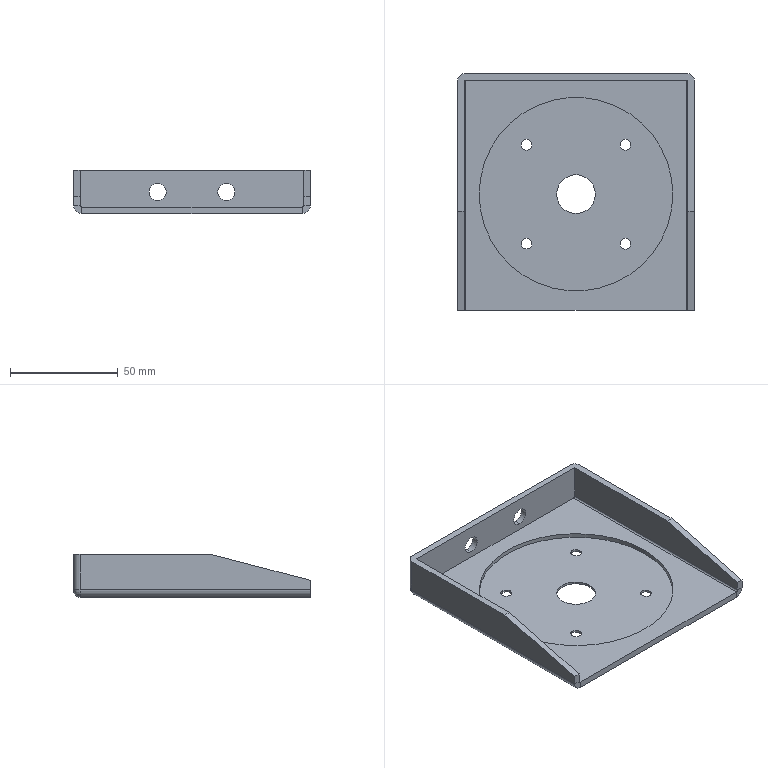Part | SolidWorks | features ICE 5, MirrorPattern 2, Cut 1, EdgeFlange 1, Fillet 1, FlatPattern 1, SMBaseFlange 1, SheetMetal 1 | 1 solid | 42 faces | box 110 x 110 x 20 mm | volume 36896 mm3 | cylinder 23 | plane 17 | torus 2 | commonest cylinder face diameters 5 x8 8 x4 6 x3 1.473 x2 7.473 x2 18 x2
STEP:
#1=CARTESIAN_POINT('',(-45.,-1.,-2.));
#2=VERTEX_POINT('',#1);
#3=CARTESIAN_POINT('',(45.,-1.,-2.));
#4=VERTEX_POINT('',#3);
#5=CARTESIAN_POINT('',(0.,-1.,-2.));
#6=DIRECTION('',(0.,0.,1.));
#7=DIRECTION('',(1.,0.,0.));
#8=AXIS2_PLACEMENT_3D('',#5,#6,#7);
#9=CIRCLE('',#8,45.);
#10=EDGE_CURVE('',#2,#4,#9,.T.);
#11=ORIENTED_EDGE('',*,*,#10,.F.);
#12=CARTESIAN_POINT('',(-45.,-1.,0.));
#13=VERTEX_POINT('',#12);
#14=CARTESIAN_POINT('',(-45.,-1.,-2.));
#15=DIRECTION('',(0.,0.,1.));
#16=VECTOR('',#15,1000.);
#17=LINE('',#14,#16);
#18=EDGE_CURVE('',#2,#13,#17,.T.);
#19=ORIENTED_EDGE('',*,*,#18,.T.);
#20=CARTESIAN_POINT('',(45.,-1.,0.));
#21=VERTEX_POINT('',#20);
#22=CARTESIAN_POINT('',(0.,-1.,0.));
#23=DIRECTION('',(0.,0.,1.));
#24=DIRECTION('',(1.,0.,0.));
#25=AXIS2_PLACEMENT_3D('',#22,#23,#24);
#26=CIRCLE('',#25,45.);
#27=EDGE_CURVE('',#13,#21,#26,.T.);
#28=ORIENTED_EDGE('',*,*,#27,.T.);
#29=CARTESIAN_POINT('',(45.,-1.,-2.));
#30=DIRECTION('',(0.,0.,1.));
#31=VECTOR('',#30,1000.);
#32=LINE('',#29,#31);
#33=EDGE_CURVE('',#4,#21,#32,.T.);
#34=ORIENTED_EDGE('',*,*,#33,.F.);
#35=EDGE_LOOP('',(#11,#19,#28,#34));
#36=FACE_OUTER_BOUND('',#35,.T.);
#37=CARTESIAN_POINT('',(0.,-1.,-2.));
#38=DIRECTION('',(0.,0.,1.));
#39=DIRECTION('',(1.,0.,0.));
#40=AXIS2_PLACEMENT_3D('',#37,#38,#39);
#41=CYLINDRICAL_SURFACE('',#40,45.);
#42=ADVANCED_FACE('',(#36),#41,.F.);
#43=CARTESIAN_POINT('',(-16.,52.,3.));
#44=VERTEX_POINT('',#43);
#45=CARTESIAN_POINT('',(-16.,52.,11.));
#46=VERTEX_POINT('',#45);
#47=CARTESIAN_POINT('',(-16.,52.,7.));
#48=DIRECTION('',(0.,1.,0.));
#49=DIRECTION('',(0.,0.,1.));
#50=AXIS2_PLACEMENT_3D('',#47,#48,#49);
#51=CIRCLE('',#50,4.);
#52=EDGE_CURVE('',#44,#46,#51,.T.);
#53=ORIENTED_EDGE('',*,*,#52,.F.);
#54=CARTESIAN_POINT('',(-16.,55.,3.));
#55=VERTEX_POINT('',#54);
#56=CARTESIAN_POINT('',(-16.,52.,3.));
#57=DIRECTION('',(0.,1.,0.));
#58=VECTOR('',#57,1000.);
#59=LINE('',#56,#58);
#60=EDGE_CURVE('',#44,#55,#59,.T.);
#61=ORIENTED_EDGE('',*,*,#60,.T.);
#62=CARTESIAN_POINT('',(-16.,55.,11.));
#63=VERTEX_POINT('',#62);
#64=CARTESIAN_POINT('',(-16.,55.,7.));
#65=DIRECTION('',(0.,1.,0.));
#66=DIRECTION('',(0.,0.,1.));
#67=AXIS2_PLACEMENT_3D('',#64,#65,#66);
#68=CIRCLE('',#67,4.);
#69=EDGE_CURVE('',#55,#63,#68,.T.);
#70=ORIENTED_EDGE('',*,*,#69,.T.);
#71=CARTESIAN_POINT('',(-16.,52.,11.));
#72=DIRECTION('',(0.,1.,0.));
#73=VECTOR('',#72,1000.);
#74=LINE('',#71,#73);
#75=EDGE_CURVE('',#46,#63,#74,.T.);
#76=ORIENTED_EDGE('',*,*,#75,.F.);
#77=EDGE_LOOP('',(#53,#61,#70,#76));
#78=FACE_OUTER_BOUND('',#77,.T.);
#79=CARTESIAN_POINT('',(-16.,52.,7.));
#80=DIRECTION('',(0.,1.,0.));
#81=DIRECTION('',(0.,0.,1.));
#82=AXIS2_PLACEMENT_3D('',#79,#80,#81);
#83=CYLINDRICAL_SURFACE('',#82,4.);
#84=ADVANCED_FACE('',(#78),#83,.F.);
#85=CARTESIAN_POINT('',(16.,52.,3.));
#86=VERTEX_POINT('',#85);
#87=CARTESIAN_POINT('',(16.,52.,11.));
#88=VERTEX_POINT('',#87);
#89=CARTESIAN_POINT('',(16.,52.,7.));
#90=DIRECTION('',(0.,1.,0.));
#91=DIRECTION('',(0.,0.,1.));
#92=AXIS2_PLACEMENT_3D('',#89,#90,#91);
#93=CIRCLE('',#92,4.);
#94=EDGE_CURVE('',#86,#88,#93,.T.);
#95=ORIENTED_EDGE('',*,*,#94,.F.);
#96=CARTESIAN_POINT('',(16.,55.,3.));
#97=VERTEX_POINT('',#96);
#98=CARTESIAN_POINT('',(16.,52.,3.));
#99=DIRECTION('',(0.,1.,0.));
#100=VECTOR('',#99,1000.);
#101=LINE('',#98,#100);
#102=EDGE_CURVE('',#86,#97,#101,.T.);
#103=ORIENTED_EDGE('',*,*,#102,.T.);
#104=CARTESIAN_POINT('',(16.,55.,11.));
#105=VERTEX_POINT('',#104);
#106=CARTESIAN_POINT('',(16.,55.,7.));
#107=DIRECTION('',(0.,1.,0.));
#108=DIRECTION('',(0.,0.,1.));
#109=AXIS2_PLACEMENT_3D('',#106,#107,#108);
#110=CIRCLE('',#109,4.);
#111=EDGE_CURVE('',#97,#105,#110,.T.);
#112=ORIENTED_EDGE('',*,*,#111,.T.);
#113=CARTESIAN_POINT('',(16.,52.,11.));
#114=DIRECTION('',(0.,1.,0.));
#115=VECTOR('',#114,1000.);
#116=LINE('',#113,#115);
#117=EDGE_CURVE('',#88,#105,#116,.T.);
#118=ORIENTED_EDGE('',*,*,#117,.F.);
#119=EDGE_LOOP('',(#95,#103,#112,#118));
#120=FACE_OUTER_BOUND('',#119,.T.);
#121=CARTESIAN_POINT('',(16.,52.,7.));
#122=DIRECTION('',(0.,1.,0.));
#123=DIRECTION('',(0.,0.,1.));
#124=AXIS2_PLACEMENT_3D('',#121,#122,#123);
#125=CYLINDRICAL_SURFACE('',#124,4.);
#126=ADVANCED_FACE('',(#120),#125,.F.);
#127=CARTESIAN_POINT('',(20.451,-24.011,-3.));
#128=VERTEX_POINT('',#127);
#129=CARTESIAN_POINT('',(25.451,-24.011,-3.));
#130=VERTEX_POINT('',#129);
#131=CARTESIAN_POINT('',(22.951,-24.011,-3.));
#132=DIRECTION('',(0.,0.,1.));
#133=DIRECTION('',(-1.,0.,0.));
#134=AXIS2_PLACEMENT_3D('',#131,#132,#133);
#135=CIRCLE('',#134,2.5);
#136=EDGE_CURVE('',#128,#130,#135,.T.);
#137=ORIENTED_EDGE('',*,*,#136,.F.);
#138=CARTESIAN_POINT('',(20.451,-24.011,-2.));
#139=VERTEX_POINT('',#138);
#140=CARTESIAN_POINT('',(20.451,-24.011,-3.));
#141=DIRECTION('',(0.,0.,1.));
#142=VECTOR('',#141,1000.);
#143=LINE('',#140,#142);
#144=EDGE_CURVE('',#128,#139,#143,.T.);
#145=ORIENTED_EDGE('',*,*,#144,.T.);
#146=CARTESIAN_POINT('',(25.451,-24.011,-2.));
#147=VERTEX_POINT('',#146);
#148=CARTESIAN_POINT('',(22.951,-24.011,-2.));
#149=DIRECTION('',(0.,0.,-1.));
#150=DIRECTION('',(1.,0.,0.));
#151=AXIS2_PLACEMENT_3D('',#148,#149,#150);
#152=CIRCLE('',#151,2.5);
#153=EDGE_CURVE('',#147,#139,#152,.T.);
#154=ORIENTED_EDGE('',*,*,#153,.F.);
#155=CARTESIAN_POINT('',(25.451,-24.011,-3.));
#156=DIRECTION('',(0.,0.,1.));
#157=VECTOR('',#156,1000.);
#158=LINE('',#155,#157);
#159=EDGE_CURVE('',#130,#147,#158,.T.);
#160=ORIENTED_EDGE('',*,*,#159,.F.);
#161=EDGE_LOOP('',(#137,#145,#154,#160));
#162=FACE_OUTER_BOUND('',#161,.T.);
#163=CARTESIAN_POINT('',(22.951,-24.011,-3.));
#164=DIRECTION('',(0.,0.,1.));
#165=DIRECTION('',(1.,0.,0.));
#166=AXIS2_PLACEMENT_3D('',#163,#164,#165);
#167=CYLINDRICAL_SURFACE('',#166,2.5);
#168=ADVANCED_FACE('',(#162),#167,.F.);
#169=CARTESIAN_POINT('',(-25.481,-23.981,-3.));
#170=VERTEX_POINT('',#169);
#171=CARTESIAN_POINT('',(-20.481,-23.981,-3.));
#172=VERTEX_POINT('',#171);
#173=CARTESIAN_POINT('',(-22.981,-23.981,-3.));
#174=DIRECTION('',(0.,0.,1.));
#175=DIRECTION('',(-1.,0.,0.));
#176=AXIS2_PLACEMENT_3D('',#173,#174,#175);
#177=CIRCLE('',#176,2.5);
#178=EDGE_CURVE('',#170,#172,#177,.T.);
#179=ORIENTED_EDGE('',*,*,#178,.F.);
#180=CARTESIAN_POINT('',(-25.481,-23.981,-2.));
#181=VERTEX_POINT('',#180);
#182=CARTESIAN_POINT('',(-25.481,-23.981,-3.));
#183=DIRECTION('',(0.,0.,1.));
#184=VECTOR('',#183,1000.);
#185=LINE('',#182,#184);
#186=EDGE_CURVE('',#170,#181,#185,.T.);
#187=ORIENTED_EDGE('',*,*,#186,.T.);
#188=CARTESIAN_POINT('',(-20.481,-23.981,-2.));
#189=VERTEX_POINT('',#188);
#190=CARTESIAN_POINT('',(-22.981,-23.981,-2.));
#191=DIRECTION('',(0.,0.,-1.));
#192=DIRECTION('',(1.,0.,0.));
#193=AXIS2_PLACEMENT_3D('',#190,#191,#192);
#194=CIRCLE('',#193,2.5);
#195=EDGE_CURVE('',#189,#181,#194,.T.);
#196=ORIENTED_EDGE('',*,*,#195,.F.);
#197=CARTESIAN_POINT('',(-20.481,-23.981,-3.));
#198=DIRECTION('',(0.,0.,1.));
#199=VECTOR('',#198,1000.);
#200=LINE('',#197,#199);
#201=EDGE_CURVE('',#172,#189,#200,.T.);
#202=ORIENTED_EDGE('',*,*,#201,.F.);
#203=EDGE_LOOP('',(#179,#187,#196,#202));
#204=FACE_OUTER_BOUND('',#203,.T.);
#205=CARTESIAN_POINT('',(-22.981,-23.981,-3.));
#206=DIRECTION('',(0.,0.,1.));
#207=DIRECTION('',(1.,0.,0.));
#208=AXIS2_PLACEMENT_3D('',#205,#206,#207);
#209=CYLINDRICAL_SURFACE('',#208,2.5);
#210=ADVANCED_FACE('',(#204),#209,.F.);
#211=CARTESIAN_POINT('',(-25.481,21.981,-3.));
#212=VERTEX_POINT('',#211);
#213=CARTESIAN_POINT('',(-20.481,21.981,-3.));
#214=VERTEX_POINT('',#213);
#215=CARTESIAN_POINT('',(-22.981,21.981,-3.));
#216=DIRECTION('',(0.,0.,1.));
#217=DIRECTION('',(1.,0.,0.));
#218=AXIS2_PLACEMENT_3D('',#215,#216,#217);
#219=CIRCLE('',#218,2.5);
#220=EDGE_CURVE('',#212,#214,#219,.T.);
#221=ORIENTED_EDGE('',*,*,#220,.F.);
#222=CARTESIAN_POINT('',(-25.481,21.981,-2.));
#223=VERTEX_POINT('',#222);
#224=CARTESIAN_POINT('',(-25.481,21.981,-3.));
#225=DIRECTION('',(0.,0.,1.));
#226=VECTOR('',#225,1000.);
#227=LINE('',#224,#226);
#228=EDGE_CURVE('',#212,#223,#227,.T.);
#229=ORIENTED_EDGE('',*,*,#228,.T.);
#230=CARTESIAN_POINT('',(-20.481,21.981,-2.));
#231=VERTEX_POINT('',#230);
#232=CARTESIAN_POINT('',(-22.981,21.981,-2.));
#233=DIRECTION('',(0.,0.,-1.));
#234=DIRECTION('',(1.,0.,0.));
#235=AXIS2_PLACEMENT_3D('',#232,#233,#234);
#236=CIRCLE('',#235,2.5);
#237=EDGE_CURVE('',#231,#223,#236,.T.);
#238=ORIENTED_EDGE('',*,*,#237,.F.);
#239=CARTESIAN_POINT('',(-20.481,21.981,-3.));
#240=DIRECTION('',(0.,0.,1.));
#241=VECTOR('',#240,1000.);
#242=LINE('',#239,#241);
#243=EDGE_CURVE('',#214,#231,#242,.T.);
#244=ORIENTED_EDGE('',*,*,#243,.F.);
#245=EDGE_LOOP('',(#221,#229,#238,#244));
#246=FACE_OUTER_BOUND('',#245,.T.);
#247=CARTESIAN_POINT('',(-22.981,21.981,-3.));
#248=DIRECTION('',(0.,0.,1.));
#249=DIRECTION('',(1.,0.,0.));
#250=AXIS2_PLACEMENT_3D('',#247,#248,#249);
#251=CYLINDRICAL_SURFACE('',#250,2.5);
#252=ADVANCED_FACE('',(#246),#251,.F.);
#253=CARTESIAN_POINT('',(20.451,22.011,-3.));
#254=VERTEX_POINT('',#253);
#255=CARTESIAN_POINT('',(25.451,22.011,-3.));
#256=VERTEX_POINT('',#255);
#257=CARTESIAN_POINT('',(22.951,22.011,-3.));
#258=DIRECTION('',(0.,0.,1.));
#259=DIRECTION('',(1.,0.,0.));
#260=AXIS2_PLACEMENT_3D('',#257,#258,#259);
#261=CIRCLE('',#260,2.5);
#262=EDGE_CURVE('',#254,#256,#261,.T.);
#263=ORIENTED_EDGE('',*,*,#262,.F.);
#264=CARTESIAN_POINT('',(20.451,22.011,-2.));
#265=VERTEX_POINT('',#264);
#266=CARTESIAN_POINT('',(20.451,22.011,-3.));
#267=DIRECTION('',(0.,0.,1.));
#268=VECTOR('',#267,1000.);
#269=LINE('',#266,#268);
#270=EDGE_CURVE('',#254,#265,#269,.T.);
#271=ORIENTED_EDGE('',*,*,#270,.T.);
#272=CARTESIAN_POINT('',(25.451,22.011,-2.));
#273=VERTEX_POINT('',#272);
#274=CARTESIAN_POINT('',(22.951,22.011,-2.));
#275=DIRECTION('',(0.,0.,-1.));
#276=DIRECTION('',(1.,0.,0.));
#277=AXIS2_PLACEMENT_3D('',#274,#275,#276);
#278=CIRCLE('',#277,2.5);
#279=EDGE_CURVE('',#273,#265,#278,.T.);
#280=ORIENTED_EDGE('',*,*,#279,.F.);
#281=CARTESIAN_POINT('',(25.451,22.011,-3.));
#282=DIRECTION('',(0.,0.,1.));
#283=VECTOR('',#282,1000.);
#284=LINE('',#281,#283);
#285=EDGE_CURVE('',#256,#273,#284,.T.);
#286=ORIENTED_EDGE('',*,*,#285,.F.);
#287=EDGE_LOOP('',(#263,#271,#280,#286));
#288=FACE_OUTER_BOUND('',#287,.T.);
#289=CARTESIAN_POINT('',(22.951,22.011,-3.));
#290=DIRECTION('',(0.,0.,1.));
#291=DIRECTION('',(1.,0.,0.));
#292=AXIS2_PLACEMENT_3D('',#289,#290,#291);
#293=CYLINDRICAL_SURFACE('',#292,2.5);
#294=ADVANCED_FACE('',(#288),#293,.F.);
#295=CARTESIAN_POINT('',(-9.,-1.,-3.));
#296=VERTEX_POINT('',#295);
#297=CARTESIAN_POINT('',(9.,-1.,-3.));
#298=VERTEX_POINT('',#297);
#299=CARTESIAN_POINT('',(0.,-1.,-3.));
#300=DIRECTION('',(0.,0.,1.));
#301=DIRECTION('',(1.,0.,0.));
#302=AXIS2_PLACEMENT_3D('',#299,#300,#301);
#303=CIRCLE('',#302,9.);
#304=EDGE_CURVE('',#296,#298,#303,.T.);
#305=ORIENTED_EDGE('',*,*,#304,.F.);
#306=CARTESIAN_POINT('',(-9.,-1.,-2.));
#307=VERTEX_POINT('',#306);
#308=CARTESIAN_POINT('',(-9.,-1.,-3.));
#309=DIRECTION('',(0.,0.,1.));
#310=VECTOR('',#309,1000.);
#311=LINE('',#308,#310);
#312=EDGE_CURVE('',#296,#307,#311,.T.);
#313=ORIENTED_EDGE('',*,*,#312,.T.);
#314=CARTESIAN_POINT('',(9.,-1.,-2.));
#315=VERTEX_POINT('',#314);
#316=CARTESIAN_POINT('',(0.,-1.,-2.));
#317=DIRECTION('',(0.,0.,-1.));
#318=DIRECTION('',(1.,0.,0.));
#319=AXIS2_PLACEMENT_3D('',#316,#317,#318);
#320=CIRCLE('',#319,9.);
#321=EDGE_CURVE('',#315,#307,#320,.T.);
#322=ORIENTED_EDGE('',*,*,#321,.F.);
#323=CARTESIAN_POINT('',(9.,-1.,-3.));
#324=DIRECTION('',(0.,0.,1.));
#325=VECTOR('',#324,1000.);
#326=LINE('',#323,#325);
#327=EDGE_CURVE('',#298,#315,#326,.T.);
#328=ORIENTED_EDGE('',*,*,#327,.F.);
#329=EDGE_LOOP('',(#305,#313,#322,#328));
#330=FACE_OUTER_BOUND('',#329,.T.);
#331=CARTESIAN_POINT('',(0.,-1.,-3.));
#332=DIRECTION('',(0.,0.,1.));
#333=DIRECTION('',(1.,0.,0.));
#334=AXIS2_PLACEMENT_3D('',#331,#332,#333);
#335=CYLINDRICAL_SURFACE('',#334,9.);
#336=ADVANCED_FACE('',(#330),#335,.F.);
#337=ORIENTED_EDGE('',*,*,#312,.F.);
#338=CARTESIAN_POINT('',(0.,-1.,-3.));
#339=DIRECTION('',(0.,0.,1.));
#340=DIRECTION('',(1.,0.,0.));
#341=AXIS2_PLACEMENT_3D('',#338,#339,#340);
#342=CIRCLE('',#341,9.);
#343=EDGE_CURVE('',#298,#296,#342,.T.);
#344=ORIENTED_EDGE('',*,*,#343,.F.);
#345=ORIENTED_EDGE('',*,*,#327,.T.);
#346=CARTESIAN_POINT('',(0.,-1.,-2.));
#347=DIRECTION('',(0.,0.,-1.));
#348=DIRECTION('',(1.,0.,0.));
#349=AXIS2_PLACEMENT_3D('',#346,#347,#348);
#350=CIRCLE('',#349,9.);
#351=EDGE_CURVE('',#307,#315,#350,.T.);
#352=ORIENTED_EDGE('',*,*,#351,.F.);
#353=EDGE_LOOP('',(#337,#344,#345,#352));
#354=FACE_OUTER_BOUND('',#353,.T.);
#355=CARTESIAN_POINT('',(0.,-1.,-3.));
#356=DIRECTION('',(0.,0.,1.));
#357=DIRECTION('',(1.,0.,0.));
#358=AXIS2_PLACEMENT_3D('',#355,#356,#357);
#359=CYLINDRICAL_SURFACE('',#358,9.);
#360=ADVANCED_FACE('',(#354),#359,.F.);
#361=ORIENTED_EDGE('',*,*,#270,.F.);
#362=CARTESIAN_POINT('',(22.951,22.011,-3.));
#363=DIRECTION('',(0.,0.,1.));
#364=DIRECTION('',(1.,0.,0.));
#365=AXIS2_PLACEMENT_3D('',#362,#363,#364);
#366=CIRCLE('',#365,2.5);
#367=EDGE_CURVE('',#256,#254,#366,.T.);
#368=ORIENTED_EDGE('',*,*,#367,.F.);
#369=ORIENTED_EDGE('',*,*,#285,.T.);
#370=CARTESIAN_POINT('',(22.951,22.011,-2.));
#371=DIRECTION('',(0.,0.,-1.));
#372=DIRECTION('',(1.,0.,0.));
#373=AXIS2_PLACEMENT_3D('',#370,#371,#372);
#374=CIRCLE('',#373,2.5);
#375=EDGE_CURVE('',#265,#273,#374,.T.);
#376=ORIENTED_EDGE('',*,*,#375,.F.);
#377=EDGE_LOOP('',(#361,#368,#369,#376));
#378=FACE_OUTER_BOUND('',#377,.T.);
#379=CARTESIAN_POINT('',(22.951,22.011,-3.));
#380=DIRECTION('',(0.,0.,1.));
#381=DIRECTION('',(1.,0.,0.));
#382=AXIS2_PLACEMENT_3D('',#379,#380,#381);
#383=CYLINDRICAL_SURFACE('',#382,2.5);
#384=ADVANCED_FACE('',(#378),#383,.F.);
#385=ORIENTED_EDGE('',*,*,#228,.F.);
#386=CARTESIAN_POINT('',(-22.981,21.981,-3.));
#387=DIRECTION('',(0.,0.,1.));
#388=DIRECTION('',(1.,0.,0.));
#389=AXIS2_PLACEMENT_3D('',#386,#387,#388);
#390=CIRCLE('',#389,2.5);
#391=EDGE_CURVE('',#214,#212,#390,.T.);
#392=ORIENTED_EDGE('',*,*,#391,.F.);
#393=ORIENTED_EDGE('',*,*,#243,.T.);
#394=CARTESIAN_POINT('',(-22.981,21.981,-2.));
#395=DIRECTION('',(0.,0.,-1.));
#396=DIRECTION('',(1.,0.,0.));
#397=AXIS2_PLACEMENT_3D('',#394,#395,#396);
#398=CIRCLE('',#397,2.5);
#399=EDGE_CURVE('',#223,#231,#398,.T.);
#400=ORIENTED_EDGE('',*,*,#399,.F.);
#401=EDGE_LOOP('',(#385,#392,#393,#400));
#402=FACE_OUTER_BOUND('',#401,.T.);
#403=CARTESIAN_POINT('',(-22.981,21.981,-3.));
#404=DIRECTION('',(0.,0.,1.));
#405=DIRECTION('',(1.,0.,0.));
#406=AXIS2_PLACEMENT_3D('',#403,#404,#405);
#407=CYLINDRICAL_SURFACE('',#406,2.5);
#408=ADVANCED_FACE('',(#402),#407,.F.);
#409=ORIENTED_EDGE('',*,*,#186,.F.);
#410=CARTESIAN_POINT('',(-22.981,-23.981,-3.));
#411=DIRECTION('',(0.,0.,1.));
#412=DIRECTION('',(-1.,0.,0.));
#413=AXIS2_PLACEMENT_3D('',#410,#411,#412);
#414=CIRCLE('',#413,2.5);
#415=EDGE_CURVE('',#172,#170,#414,.T.);
#416=ORIENTED_EDGE('',*,*,#415,.F.);
#417=ORIENTED_EDGE('',*,*,#201,.T.);
#418=CARTESIAN_POINT('',(-22.981,-23.981,-2.));
#419=DIRECTION('',(0.,0.,-1.));
#420=DIRECTION('',(1.,0.,0.));
#421=AXIS2_PLACEMENT_3D('',#418,#419,#420);
#422=CIRCLE('',#421,2.5);
#423=EDGE_CURVE('',#181,#189,#422,.T.);
#424=ORIENTED_EDGE('',*,*,#423,.F.);
#425=EDGE_LOOP('',(#409,#416,#417,#424));
#426=FACE_OUTER_BOUND('',#425,.T.);
#427=CARTESIAN_POINT('',(-22.981,-23.981,-3.));
#428=DIRECTION('',(0.,0.,1.));
#429=DIRECTION('',(1.,0.,0.));
#430=AXIS2_PLACEMENT_3D('',#427,#428,#429);
#431=CYLINDRICAL_SURFACE('',#430,2.5);
#432=ADVANCED_FACE('',(#426),#431,.F.);
#433=ORIENTED_EDGE('',*,*,#144,.F.);
#434=CARTESIAN_POINT('',(22.951,-24.011,-3.));
#435=DIRECTION('',(0.,0.,1.));
#436=DIRECTION('',(-1.,0.,0.));
#437=AXIS2_PLACEMENT_3D('',#434,#435,#436);
#438=CIRCLE('',#437,2.5);
#439=EDGE_CURVE('',#130,#128,#438,.T.);
#440=ORIENTED_EDGE('',*,*,#439,.F.);
#441=ORIENTED_EDGE('',*,*,#159,.T.);
#442=CARTESIAN_POINT('',(22.951,-24.011,-2.));
#443=DIRECTION('',(0.,0.,-1.));
#444=DIRECTION('',(1.,0.,0.));
#445=AXIS2_PLACEMENT_3D('',#442,#443,#444);
#446=CIRCLE('',#445,2.5);
#447=EDGE_CURVE('',#139,#147,#446,.T.);
#448=ORIENTED_EDGE('',*,*,#447,.F.);
#449=EDGE_LOOP('',(#433,#440,#441,#448));
#450=FACE_OUTER_BOUND('',#449,.T.);
#451=CARTESIAN_POINT('',(22.951,-24.011,-3.));
#452=DIRECTION('',(0.,0.,1.));
#453=DIRECTION('',(1.,0.,0.));
#454=AXIS2_PLACEMENT_3D('',#451,#452,#453);
#455=CYLINDRICAL_SURFACE('',#454,2.5);
#456=ADVANCED_FACE('',(#450),#455,.F.);
#457=CARTESIAN_POINT('',(-52.,52.,17.));
#458=VERTEX_POINT('',#457);
#459=CARTESIAN_POINT('',(-52.,-9.,17.));
#460=VERTEX_POINT('',#459);
#461=CARTESIAN_POINT('',(-52.,0.,17.));
#462=DIRECTION('',(0.,-1.,0.));
#463=VECTOR('',#462,1000.);
#464=LINE('',#461,#463);
#465=EDGE_CURVE('',#458,#460,#464,.T.);
#466=ORIENTED_EDGE('',*,*,#465,.T.);
#467=CARTESIAN_POINT('',(-52.,-55.,5.));
#468=VERTEX_POINT('',#467);
#469=CARTESIAN_POINT('',(-52.,-4.726,18.115));
#470=DIRECTION('',(0.,-0.9676,-0.2524));
#471=VECTOR('',#470,1000.);
#472=LINE('',#469,#471);
#473=EDGE_CURVE('',#460,#468,#472,.T.);
#474=ORIENTED_EDGE('',*,*,#473,.T.);
#475=CARTESIAN_POINT('',(-52.,-55.,0.7366));
#476=VERTEX_POINT('',#475);
#477=CARTESIAN_POINT('',(-52.,-55.,0.));
#478=DIRECTION('',(0.,0.,-1.));
#479=VECTOR('',#478,1000.);
#480=LINE('',#477,#479);
#481=EDGE_CURVE('',#468,#476,#480,.T.);
#482=ORIENTED_EDGE('',*,*,#481,.T.);
#483=CARTESIAN_POINT('',(-52.,52.,0.7366));
#484=VERTEX_POINT('',#483);
#485=CARTESIAN_POINT('',(-52.,55.,0.7366));
#486=DIRECTION('',(0.,-1.,0.));
#487=VECTOR('',#486,1000.);
#488=LINE('',#485,#487);
#489=EDGE_CURVE('',#484,#476,#488,.T.);
#490=ORIENTED_EDGE('',*,*,#489,.F.);
#491=CARTESIAN_POINT('',(-52.,52.,0.7366));
#492=DIRECTION('',(0.,0.,1.));
#493=VECTOR('',#492,1000.);
#494=LINE('',#491,#493);
#495=EDGE_CURVE('',#484,#458,#494,.T.);
#496=ORIENTED_EDGE('',*,*,#495,.T.);
#497=EDGE_LOOP('',(#466,#474,#482,#490,#496));
#498=FACE_OUTER_BOUND('',#497,.T.);
#499=CARTESIAN_POINT('',(-52.,0.,0.));
#500=DIRECTION('',(1.,0.,0.));
#501=DIRECTION('',(0.,0.,1.));
#502=AXIS2_PLACEMENT_3D('',#499,#500,#501);
#503=PLANE('',#502);
#504=ADVANCED_FACE('',(#498),#503,.T.);
#505=CARTESIAN_POINT('',(-55.,-9.,17.));
#506=VERTEX_POINT('',#505);
#507=CARTESIAN_POINT('',(-45.,-9.,17.));
#508=DIRECTION('',(-1.,0.,0.));
#509=VECTOR('',#508,1000.);
#510=LINE('',#507,#509);
#511=EDGE_CURVE('',#460,#506,#510,.T.);
#512=ORIENTED_EDGE('',*,*,#511,.F.);
#513=ORIENTED_EDGE('',*,*,#465,.F.);
#514=CARTESIAN_POINT('',(52.,52.,17.));
#515=VERTEX_POINT('',#514);
#516=CARTESIAN_POINT('',(-52.,52.,17.));
#517=DIRECTION('',(1.,0.,0.));
#518=VECTOR('',#517,1000.);
#519=LINE('',#516,#518);
#520=EDGE_CURVE('',#458,#515,#519,.T.);
#521=ORIENTED_EDGE('',*,*,#520,.T.);
#522=CARTESIAN_POINT('',(52.,-9.,17.));
#523=VERTEX_POINT('',#522);
#524=CARTESIAN_POINT('',(52.,-55.,17.));
#525=DIRECTION('',(0.,-1.,0.));
#526=VECTOR('',#525,1000.);
#527=LINE('',#524,#526);
#528=EDGE_CURVE('',#515,#523,#527,.T.);
#529=ORIENTED_EDGE('',*,*,#528,.T.);
#530=CARTESIAN_POINT('',(55.,-9.,17.));
#531=VERTEX_POINT('',#530);
#532=CARTESIAN_POINT('',(55.,-9.,17.));
#533=DIRECTION('',(1.,0.,0.));
#534=VECTOR('',#533,1000.);
#535=LINE('',#532,#534);
#536=EDGE_CURVE('',#523,#531,#535,.T.);
#537=ORIENTED_EDGE('',*,*,#536,.T.);
#538=CARTESIAN_POINT('',(55.,52.,17.));
#539=VERTEX_POINT('',#538);
#540=CARTESIAN_POINT('',(55.,0.,17.));
#541=DIRECTION('',(0.,-1.,0.));
#542=VECTOR('',#541,1000.);
#543=LINE('',#540,#542);
#544=EDGE_CURVE('',#539,#531,#543,.T.);
#545=ORIENTED_EDGE('',*,*,#544,.F.);
#546=CARTESIAN_POINT('',(52.,55.,17.));
#547=VERTEX_POINT('',#546);
#548=CARTESIAN_POINT('',(52.,52.,17.));
#549=DIRECTION('',(0.,0.,1.));
#550=DIRECTION('',(-1.,0.,0.));
#551=AXIS2_PLACEMENT_3D('',#548,#549,#550);
#552=CIRCLE('',#551,3.);
#553=EDGE_CURVE('',#539,#547,#552,.T.);
#554=ORIENTED_EDGE('',*,*,#553,.T.);
#555=CARTESIAN_POINT('',(-52.,55.,17.));
#556=VERTEX_POINT('',#555);
#557=CARTESIAN_POINT('',(55.,55.,17.));
#558=DIRECTION('',(-1.,0.,0.));
#559=VECTOR('',#558,1000.);
#560=LINE('',#557,#559);
#561=EDGE_CURVE('',#547,#556,#560,.T.);
#562=ORIENTED_EDGE('',*,*,#561,.T.);
#563=CARTESIAN_POINT('',(-55.,52.,17.));
#564=VERTEX_POINT('',#563);
#565=CARTESIAN_POINT('',(-52.,52.,17.));
#566=DIRECTION('',(0.,0.,1.));
#567=DIRECTION('',(-1.,0.,0.));
#568=AXIS2_PLACEMENT_3D('',#565,#566,#567);
#569=CIRCLE('',#568,3.);
#570=EDGE_CURVE('',#556,#564,#569,.T.);
#571=ORIENTED_EDGE('',*,*,#570,.T.);
#572=CARTESIAN_POINT('',(-55.,-55.,17.));
#573=DIRECTION('',(0.,-1.,0.));
#574=VECTOR('',#573,1000.);
#575=LINE('',#572,#574);
#576=EDGE_CURVE('',#564,#506,#575,.T.);
#577=ORIENTED_EDGE('',*,*,#576,.T.);
#578=EDGE_LOOP('',(#512,#513,#521,#529,#537,#545,#554,#562,#571,#577));
#579=FACE_OUTER_BOUND('',#578,.T.);
#580=CARTESIAN_POINT('',(55.,-55.,17.));
#581=DIRECTION('',(0.,0.,-1.));
#582=DIRECTION('',(-1.,0.,0.));
#583=AXIS2_PLACEMENT_3D('',#580,#581,#582);
#584=PLANE('',#583);
#585=ADVANCED_FACE('',(#579),#584,.F.);
#586=ORIENTED_EDGE('',*,*,#481,.F.);
#587=CARTESIAN_POINT('',(-55.,-55.,5.));
#588=VERTEX_POINT('',#587);
#589=CARTESIAN_POINT('',(-45.,-55.,5.));
#590=DIRECTION('',(-1.,0.,0.));
#591=VECTOR('',#590,1000.);
#592=LINE('',#589,#591);
#593=EDGE_CURVE('',#468,#588,#592,.T.);
#594=ORIENTED_EDGE('',*,*,#593,.T.);
#595=CARTESIAN_POINT('',(-55.,-55.,0.7366));
#596=VERTEX_POINT('',#595);
#597=CARTESIAN_POINT('',(-55.,-55.,0.));
#598=DIRECTION('',(0.,0.,-1.));
#599=VECTOR('',#598,1000.);
#600=LINE('',#597,#599);
#601=EDGE_CURVE('',#588,#596,#600,.T.);
#602=ORIENTED_EDGE('',*,*,#601,.T.);
#603=CARTESIAN_POINT('',(-52.,-55.,0.7366));
#604=DIRECTION('',(-1.,0.,0.));
#605=VECTOR('',#604,1000.);
#606=LINE('',#603,#605);
#607=EDGE_CURVE('',#476,#596,#606,.T.);
#608=ORIENTED_EDGE('',*,*,#607,.F.);
#609=EDGE_LOOP('',(#586,#594,#602,#608));
#610=FACE_OUTER_BOUND('',#609,.T.);
#611=CARTESIAN_POINT('',(-55.,-55.,0.));
#612=DIRECTION('',(0.,-1.,0.));
#613=DIRECTION('',(0.,0.,-1.));
#614=AXIS2_PLACEMENT_3D('',#611,#612,#613);
#615=PLANE('',#614);
#616=ADVANCED_FACE('',(#610),#615,.T.);
#617=CARTESIAN_POINT('',(-55.,-55.,5.));
#618=DIRECTION('',(0.,0.9676,0.2524));
#619=VECTOR('',#618,1000.);
#620=LINE('',#617,#619);
#621=EDGE_CURVE('',#588,#506,#620,.T.);
#622=ORIENTED_EDGE('',*,*,#621,.T.);
#623=ORIENTED_EDGE('',*,*,#576,.F.);
#624=CARTESIAN_POINT('',(-55.,52.,0.7366));
#625=VERTEX_POINT('',#624);
#626=CARTESIAN_POINT('',(-55.,52.,0.7366));
#627=DIRECTION('',(0.,0.,-1.));
#628=VECTOR('',#627,1000.);
#629=LINE('',#626,#628);
#630=EDGE_CURVE('',#564,#625,#629,.T.);
#631=ORIENTED_EDGE('',*,*,#630,.T.);
#632=CARTESIAN_POINT('',(-55.,55.,0.7366));
#633=DIRECTION('',(0.,1.,0.));
#634=VECTOR('',#633,1000.);
#635=LINE('',#632,#634);
#636=EDGE_CURVE('',#596,#625,#635,.T.);
#637=ORIENTED_EDGE('',*,*,#636,.F.);
#638=ORIENTED_EDGE('',*,*,#601,.F.);
#639=EDGE_LOOP('',(#622,#623,#631,#637,#638));
#640=FACE_OUTER_BOUND('',#639,.T.);
#641=CARTESIAN_POINT('',(-55.,0.,0.));
#642=DIRECTION('',(1.,0.,0.));
#643=DIRECTION('',(0.,0.,1.));
#644=AXIS2_PLACEMENT_3D('',#641,#642,#643);
#645=PLANE('',#644);
#646=ADVANCED_FACE('',(#640),#645,.F.);
#647=CARTESIAN_POINT('',(0.,-1.,0.));
#648=DIRECTION('',(0.,0.,1.));
#649=DIRECTION('',(1.,0.,0.));
#650=AXIS2_PLACEMENT_3D('',#647,#648,#649);
#651=CIRCLE('',#650,45.);
#652=EDGE_CURVE('',#21,#13,#651,.T.);
#653=ORIENTED_EDGE('',*,*,#652,.F.);
#654=ORIENTED_EDGE('',*,*,#27,.F.);
#655=EDGE_LOOP('',(#653,#654));
#656=FACE_BOUND('',#655,.T.);
#657=CARTESIAN_POINT('',(51.263,52.,0.));
#658=VERTEX_POINT('',#657);
#659=CARTESIAN_POINT('',(-51.263,52.,0.));
#660=VERTEX_POINT('',#659);
#661=CARTESIAN_POINT('',(51.263,52.,0.));
#662=DIRECTION('',(-1.,0.,0.));
#663=VECTOR('',#662,1000.);
#664=LINE('',#661,#663);
#665=EDGE_CURVE('',#658,#660,#664,.T.);
#666=ORIENTED_EDGE('',*,*,#665,.T.);
#667=CARTESIAN_POINT('',(-51.263,-55.,0.));
#668=VERTEX_POINT('',#667);
#669=CARTESIAN_POINT('',(-51.263,-55.,0.));
#670=DIRECTION('',(0.,1.,0.));
#671=VECTOR('',#670,1000.);
#672=LINE('',#669,#671);
#673=EDGE_CURVE('',#668,#660,#672,.T.);
#674=ORIENTED_EDGE('',*,*,#673,.F.);
#675=CARTESIAN_POINT('',(51.263,-55.,0.));
#676=VERTEX_POINT('',#675);
#677=CARTESIAN_POINT('',(-55.,-55.,0.));
#678=DIRECTION('',(1.,0.,0.));
#679=VECTOR('',#678,1000.);
#680=LINE('',#677,#679);
#681=EDGE_CURVE('',#668,#676,#680,.T.);
#682=ORIENTED_EDGE('',*,*,#681,.T.);
#683=CARTESIAN_POINT('',(51.263,55.,0.));
#684=DIRECTION('',(0.,-1.,0.));
#685=VECTOR('',#684,1000.);
#686=LINE('',#683,#685);
#687=EDGE_CURVE('',#658,#676,#686,.T.);
#688=ORIENTED_EDGE('',*,*,#687,.F.);
#689=EDGE_LOOP('',(#666,#674,#682,#688));
#690=FACE_OUTER_BOUND('',#689,.T.);
#691=CARTESIAN_POINT('',(0.,0.,0.));
#692=DIRECTION('',(0.,0.,-1.));
#693=DIRECTION('',(-1.,0.,0.));
#694=AXIS2_PLACEMENT_3D('',#691,#692,#693);
#695=PLANE('',#694);
#696=ADVANCED_FACE('',(#656,#690),#695,.F.);
#697=CARTESIAN_POINT('',(52.,52.,0.7366));
#698=VERTEX_POINT('',#697);
#699=CARTESIAN_POINT('',(51.263,52.,0.7366));
#700=DIRECTION('',(0.,1.,0.));
#701=DIRECTION('',(0.,0.,1.));
#702=AXIS2_PLACEMENT_3D('',#699,#700,#701);
#703=CIRCLE('',#702,0.7366);
#704=EDGE_CURVE('',#698,#658,#703,.T.);
#705=ORIENTED_EDGE('',*,*,#704,.T.);
#706=ORIENTED_EDGE('',*,*,#687,.T.);
#707=CARTESIAN_POINT('',(52.,-55.,0.7366));
#708=VERTEX_POINT('',#707);
#709=CARTESIAN_POINT('',(51.263,-55.,0.7366));
#710=DIRECTION('',(0.,-1.,0.));
#711=DIRECTION('',(0.,0.,1.));
#712=AXIS2_PLACEMENT_3D('',#709,#710,#711);
#713=CIRCLE('',#712,0.7366);
#714=EDGE_CURVE('',#676,#708,#713,.T.);
#715=ORIENTED_EDGE('',*,*,#714,.T.);
#716=CARTESIAN_POINT('',(52.,-55.,0.7366));
#717=DIRECTION('',(0.,1.,0.));
#718=VECTOR('',#717,1000.);
#719=LINE('',#716,#718);
#720=EDGE_CURVE('',#708,#698,#719,.T.);
#721=ORIENTED_EDGE('',*,*,#720,.T.);
#722=EDGE_LOOP('',(#705,#706,#715,#721));
#723=FACE_OUTER_BOUND('',#722,.T.);
#724=CARTESIAN_POINT('',(51.263,55.,0.7366));
#725=DIRECTION('',(0.,1.,0.));
#726=DIRECTION('',(1.,0.,0.));
#727=AXIS2_PLACEMENT_3D('',#724,#725,#726);
#728=CYLINDRICAL_SURFACE('',#727,0.7366);
#729=ADVANCED_FACE('',(#723),#728,.F.);
#730=ORIENTED_EDGE('',*,*,#528,.F.);
#731=CARTESIAN_POINT('',(52.,52.,0.7366));
#732=DIRECTION('',(0.,0.,-1.));
#733=VECTOR('',#732,1000.);
#734=LINE('',#731,#733);
#735=EDGE_CURVE('',#515,#698,#734,.T.);
#736=ORIENTED_EDGE('',*,*,#735,.T.);
#737=ORIENTED_EDGE('',*,*,#720,.F.);
#738=CARTESIAN_POINT('',(52.,-55.,5.));
#739=VERTEX_POINT('',#738);
#740=CARTESIAN_POINT('',(52.,-55.,0.));
#741=DIRECTION('',(0.,0.,-1.));
#742=VECTOR('',#741,1000.);
#743=LINE('',#740,#742);
#744=EDGE_CURVE('',#739,#708,#743,.T.);
#745=ORIENTED_EDGE('',*,*,#744,.F.);
#746=CARTESIAN_POINT('',(52.,-4.726,18.115));
#747=DIRECTION('',(0.,-0.9676,-0.2524));
#748=VECTOR('',#747,1000.);
#749=LINE('',#746,#748);
#750=EDGE_CURVE('',#523,#739,#749,.T.);
#751=ORIENTED_EDGE('',*,*,#750,.F.);
#752=EDGE_LOOP('',(#730,#736,#737,#745,#751));
#753=FACE_OUTER_BOUND('',#752,.T.);
#754=CARTESIAN_POINT('',(52.,0.,0.));
#755=DIRECTION('',(-1.,0.,0.));
#756=DIRECTION('',(0.,0.,1.));
#757=AXIS2_PLACEMENT_3D('',#754,#755,#756);
#758=PLANE('',#757);
#759=ADVANCED_FACE('',(#753),#758,.T.);
#760=CARTESIAN_POINT('',(-51.263,52.,0.7366));
#761=DIRECTION('',(0.,1.,0.));
#762=DIRECTION('',(0.,0.,1.));
#763=AXIS2_PLACEMENT_3D('',#760,#761,#762);
#764=CIRCLE('',#763,0.7366);
#765=EDGE_CURVE('',#660,#484,#764,.T.);
#766=ORIENTED_EDGE('',*,*,#765,.T.);
#767=ORIENTED_EDGE('',*,*,#489,.T.);
#768=CARTESIAN_POINT('',(-51.263,-55.,0.7366));
#769=DIRECTION('',(0.,-1.,0.));
#770=DIRECTION('',(0.,0.,-1.));
#771=AXIS2_PLACEMENT_3D('',#768,#769,#770);
#772=CIRCLE('',#771,0.7366);
#773=EDGE_CURVE('',#476,#668,#772,.T.);
#774=ORIENTED_EDGE('',*,*,#773,.T.);
#775=ORIENTED_EDGE('',*,*,#673,.T.);
#776=EDGE_LOOP('',(#766,#767,#774,#775));
#777=FACE_OUTER_BOUND('',#776,.T.);
#778=CARTESIAN_POINT('',(-51.263,-55.,0.7366));
#779=DIRECTION('',(0.,-1.,0.));
#780=DIRECTION('',(-1.,0.,0.));
#781=AXIS2_PLACEMENT_3D('',#778,#779,#780);
#782=CYLINDRICAL_SURFACE('',#781,0.7366);
#783=ADVANCED_FACE('',(#777),#782,.F.);
#784=ORIENTED_EDGE('',*,*,#439,.T.);
#785=ORIENTED_EDGE('',*,*,#136,.T.);
#786=EDGE_LOOP('',(#784,#785));
#787=FACE_BOUND('',#786,.T.);
#788=ORIENTED_EDGE('',*,*,#415,.T.);
#789=ORIENTED_EDGE('',*,*,#178,.T.);
#790=EDGE_LOOP('',(#788,#789));
#791=FACE_BOUND('',#790,.T.);
#792=ORIENTED_EDGE('',*,*,#391,.T.);
#793=ORIENTED_EDGE('',*,*,#220,.T.);
#794=EDGE_LOOP('',(#792,#793));
#795=FACE_BOUND('',#794,.T.);
#796=ORIENTED_EDGE('',*,*,#367,.T.);
#797=ORIENTED_EDGE('',*,*,#262,.T.);
#798=EDGE_LOOP('',(#796,#797));
#799=FACE_BOUND('',#798,.T.);
#800=ORIENTED_EDGE('',*,*,#343,.T.);
#801=ORIENTED_EDGE('',*,*,#304,.T.);
#802=EDGE_LOOP('',(#800,#801));
#803=FACE_BOUND('',#802,.T.);
#804=CARTESIAN_POINT('',(-51.263,-55.,-3.));
#805=VERTEX_POINT('',#804);
#806=CARTESIAN_POINT('',(-51.263,52.,-3.));
#807=VERTEX_POINT('',#806);
#808=CARTESIAN_POINT('',(-51.263,-55.,-3.));
#809=DIRECTION('',(0.,1.,0.));
#810=VECTOR('',#809,1000.);
#811=LINE('',#808,#810);
#812=EDGE_CURVE('',#805,#807,#811,.T.);
#813=ORIENTED_EDGE('',*,*,#812,.T.);
#814=CARTESIAN_POINT('',(51.263,52.,-3.));
#815=VERTEX_POINT('',#814);
#816=CARTESIAN_POINT('',(0.,52.,-3.));
#817=DIRECTION('',(1.,0.,0.));
#818=VECTOR('',#817,1000.);
#819=LINE('',#816,#818);
#820=EDGE_CURVE('',#807,#815,#819,.T.);
#821=ORIENTED_EDGE('',*,*,#820,.T.);
#822=CARTESIAN_POINT('',(51.263,-55.,-3.));
#823=VERTEX_POINT('',#822);
#824=CARTESIAN_POINT('',(51.263,55.,-3.));
#825=DIRECTION('',(0.,-1.,0.));
#826=VECTOR('',#825,1000.);
#827=LINE('',#824,#826);
#828=EDGE_CURVE('',#815,#823,#827,.T.);
#829=ORIENTED_EDGE('',*,*,#828,.T.);
#830=CARTESIAN_POINT('',(-55.,-55.,-3.));
#831=DIRECTION('',(1.,0.,0.));
#832=VECTOR('',#831,1000.);
#833=LINE('',#830,#832);
#834=EDGE_CURVE('',#805,#823,#833,.T.);
#835=ORIENTED_EDGE('',*,*,#834,.F.);
#836=EDGE_LOOP('',(#813,#821,#829,#835));
#837=FACE_OUTER_BOUND('',#836,.T.);
#838=CARTESIAN_POINT('',(0.,0.,-3.));
#839=DIRECTION('',(0.,0.,-1.));
#840=DIRECTION('',(-1.,0.,0.));
#841=AXIS2_PLACEMENT_3D('',#838,#839,#840);
#842=PLANE('',#841);
#843=ADVANCED_FACE('',(#787,#791,#795,#799,#803,#837),#842,.T.);
#844=ORIENTED_EDGE('',*,*,#681,.F.);
#845=CARTESIAN_POINT('',(-51.263,-55.,0.));
#846=DIRECTION('',(0.,0.,-1.));
#847=VECTOR('',#846,1000.);
#848=LINE('',#845,#847);
#849=EDGE_CURVE('',#668,#805,#848,.T.);
#850=ORIENTED_EDGE('',*,*,#849,.T.);
#851=ORIENTED_EDGE('',*,*,#834,.T.);
#852=CARTESIAN_POINT('',(51.263,-55.,0.));
#853=DIRECTION('',(0.,0.,-1.));
#854=VECTOR('',#853,1000.);
#855=LINE('',#852,#854);
#856=EDGE_CURVE('',#676,#823,#855,.T.);
#857=ORIENTED_EDGE('',*,*,#856,.F.);
#858=EDGE_LOOP('',(#844,#850,#851,#857));
#859=FACE_OUTER_BOUND('',#858,.T.);
#860=CARTESIAN_POINT('',(-55.,-55.,-3.));
#861=DIRECTION('',(0.,-1.,0.));
#862=DIRECTION('',(0.,0.,-1.));
#863=AXIS2_PLACEMENT_3D('',#860,#861,#862);
#864=PLANE('',#863);
#865=ADVANCED_FACE('',(#859),#864,.T.);
#866=CARTESIAN_POINT('',(-16.,55.,7.));
#867=DIRECTION('',(0.,1.,0.));
#868=DIRECTION('',(0.,0.,1.));
#869=AXIS2_PLACEMENT_3D('',#866,#867,#868);
#870=CIRCLE('',#869,4.);
#871=EDGE_CURVE('',#63,#55,#870,.T.);
#872=ORIENTED_EDGE('',*,*,#871,.F.);
#873=ORIENTED_EDGE('',*,*,#69,.F.);
#874=EDGE_LOOP('',(#872,#873));
#875=FACE_BOUND('',#874,.T.);
#876=CARTESIAN_POINT('',(16.,55.,7.));
#877=DIRECTION('',(0.,1.,0.));
#878=DIRECTION('',(0.,0.,1.));
#879=AXIS2_PLACEMENT_3D('',#876,#877,#878);
#880=CIRCLE('',#879,4.);
#881=EDGE_CURVE('',#105,#97,#880,.T.);
#882=ORIENTED_EDGE('',*,*,#881,.F.);
#883=ORIENTED_EDGE('',*,*,#111,.F.);
#884=EDGE_LOOP('',(#882,#883));
#885=FACE_BOUND('',#884,.T.);
#886=ORIENTED_EDGE('',*,*,#561,.F.);
#887=CARTESIAN_POINT('',(52.,55.,0.7366));
#888=VERTEX_POINT('',#887);
#889=CARTESIAN_POINT('',(52.,55.,0.7366));
#890=DIRECTION('',(0.,0.,-1.));
#891=VECTOR('',#890,1000.);
#892=LINE('',#889,#891);
#893=EDGE_CURVE('',#547,#888,#892,.T.);
#894=ORIENTED_EDGE('',*,*,#893,.T.);
#895=CARTESIAN_POINT('',(51.263,55.,0.));
#896=VERTEX_POINT('',#895);
#897=CARTESIAN_POINT('',(51.263,55.,0.7366));
#898=DIRECTION('',(0.,1.,0.));
#899=DIRECTION('',(0.,0.,1.));
#900=AXIS2_PLACEMENT_3D('',#897,#898,#899);
#901=CIRCLE('',#900,0.7366);
#902=EDGE_CURVE('',#888,#896,#901,.T.);
#903=ORIENTED_EDGE('',*,*,#902,.T.);
#904=CARTESIAN_POINT('',(-51.263,55.,0.));
#905=VERTEX_POINT('',#904);
#906=CARTESIAN_POINT('',(-55.,55.,0.));
#907=DIRECTION('',(-1.,0.,0.));
#908=VECTOR('',#907,1000.);
#909=LINE('',#906,#908);
#910=EDGE_CURVE('',#896,#905,#909,.T.);
#911=ORIENTED_EDGE('',*,*,#910,.T.);
#912=CARTESIAN_POINT('',(-52.,55.,0.7366));
#913=VERTEX_POINT('',#912);
#914=CARTESIAN_POINT('',(-51.263,55.,0.7366));
#915=DIRECTION('',(0.,1.,0.));
#916=DIRECTION('',(0.,0.,1.));
#917=AXIS2_PLACEMENT_3D('',#914,#915,#916);
#918=CIRCLE('',#917,0.7366);
#919=EDGE_CURVE('',#905,#913,#918,.T.);
#920=ORIENTED_EDGE('',*,*,#919,.T.);
#921=CARTESIAN_POINT('',(-52.,55.,17.));
#922=DIRECTION('',(0.,0.,1.));
#923=VECTOR('',#922,1000.);
#924=LINE('',#921,#923);
#925=EDGE_CURVE('',#913,#556,#924,.T.);
#926=ORIENTED_EDGE('',*,*,#925,.T.);
#927=EDGE_LOOP('',(#886,#894,#903,#911,#920,#926));
#928=FACE_OUTER_BOUND('',#927,.T.);
#929=CARTESIAN_POINT('',(-55.,55.,-3.));
#930=DIRECTION('',(0.,1.,0.));
#931=DIRECTION('',(0.,0.,1.));
#932=AXIS2_PLACEMENT_3D('',#929,#930,#931);
#933=PLANE('',#932);
#934=ADVANCED_FACE('',(#875,#885,#928),#933,.T.);
#935=CARTESIAN_POINT('',(55.,-55.,0.7366));
#936=VERTEX_POINT('',#935);
#937=CARTESIAN_POINT('',(55.,-55.,0.7366));
#938=DIRECTION('',(1.,0.,0.));
#939=VECTOR('',#938,1000.);
#940=LINE('',#937,#939);
#941=EDGE_CURVE('',#708,#936,#940,.T.);
#942=ORIENTED_EDGE('',*,*,#941,.F.);
#943=ORIENTED_EDGE('',*,*,#714,.F.);
#944=ORIENTED_EDGE('',*,*,#856,.T.);
#945=CARTESIAN_POINT('',(51.263,-55.,0.7366));
#946=DIRECTION('',(0.,-1.,0.));
#947=DIRECTION('',(0.,0.,1.));
#948=AXIS2_PLACEMENT_3D('',#945,#946,#947);
#949=CIRCLE('',#948,3.737);
#950=EDGE_CURVE('',#823,#936,#949,.T.);
#951=ORIENTED_EDGE('',*,*,#950,.T.);
#952=EDGE_LOOP('',(#942,#943,#944,#951));
#953=FACE_OUTER_BOUND('',#952,.T.);
#954=CARTESIAN_POINT('',(51.263,-55.,0.7366));
#955=DIRECTION('',(0.,-1.,0.));
#956=DIRECTION('',(0.,0.,-1.));
#957=AXIS2_PLACEMENT_3D('',#954,#955,#956);
#958=PLANE('',#957);
#959=ADVANCED_FACE('',(#953),#958,.T.);
#960=ORIENTED_EDGE('',*,*,#828,.F.);
#961=CARTESIAN_POINT('',(55.,52.,0.7366));
#962=VERTEX_POINT('',#961);
#963=CARTESIAN_POINT('',(51.263,52.,0.7366));
#964=DIRECTION('',(0.,-1.,0.));
#965=DIRECTION('',(0.,0.,1.));
#966=AXIS2_PLACEMENT_3D('',#963,#964,#965);
#967=CIRCLE('',#966,3.737);
#968=EDGE_CURVE('',#815,#962,#967,.T.);
#969=ORIENTED_EDGE('',*,*,#968,.T.);
#970=CARTESIAN_POINT('',(55.,-55.,0.7366));
#971=DIRECTION('',(0.,-1.,0.));
#972=VECTOR('',#971,1000.);
#973=LINE('',#970,#972);
#974=EDGE_CURVE('',#962,#936,#973,.T.);
#975=ORIENTED_EDGE('',*,*,#974,.T.);
#976=ORIENTED_EDGE('',*,*,#950,.F.);
#977=EDGE_LOOP('',(#960,#969,#975,#976));
#978=FACE_OUTER_BOUND('',#977,.T.);
#979=CARTESIAN_POINT('',(51.263,55.,0.7366));
#980=DIRECTION('',(0.,1.,0.));
#981=DIRECTION('',(1.,0.,0.));
#982=AXIS2_PLACEMENT_3D('',#979,#980,#981);
#983=CYLINDRICAL_SURFACE('',#982,3.737);
#984=ADVANCED_FACE('',(#978),#983,.T.);
#985=CARTESIAN_POINT('',(55.,-55.,5.));
#986=VERTEX_POINT('',#985);
#987=CARTESIAN_POINT('',(55.,-55.,0.));
#988=DIRECTION('',(0.,0.,-1.));
#989=VECTOR('',#988,1000.);
#990=LINE('',#987,#989);
#991=EDGE_CURVE('',#986,#936,#990,.T.);
#992=ORIENTED_EDGE('',*,*,#991,.F.);
#993=CARTESIAN_POINT('',(45.,-55.,5.));
#994=DIRECTION('',(1.,0.,0.));
#995=VECTOR('',#994,1000.);
#996=LINE('',#993,#995);
#997=EDGE_CURVE('',#739,#986,#996,.T.);
#998=ORIENTED_EDGE('',*,*,#997,.F.);
#999=ORIENTED_EDGE('',*,*,#744,.T.);
#1000=ORIENTED_EDGE('',*,*,#941,.T.);
#1001=EDGE_LOOP('',(#992,#998,#999,#1000));
#1002=FACE_OUTER_BOUND('',#1001,.T.);
#1003=CARTESIAN_POINT('',(55.,-55.,0.));
#1004=DIRECTION('',(0.,1.,0.));
#1005=DIRECTION('',(0.,0.,1.));
#1006=AXIS2_PLACEMENT_3D('',#1003,#1004,#1005);
#1007=PLANE('',#1006);
#1008=ADVANCED_FACE('',(#1002),#1007,.F.);
#1009=ORIENTED_EDGE('',*,*,#974,.F.);
#1010=CARTESIAN_POINT('',(55.,52.,17.));
#1011=DIRECTION('',(0.,0.,1.));
#1012=VECTOR('',#1011,1000.);
#1013=LINE('',#1010,#1012);
#1014=EDGE_CURVE('',#962,#539,#1013,.T.);
#1015=ORIENTED_EDGE('',*,*,#1014,.T.);
#1016=ORIENTED_EDGE('',*,*,#544,.T.);
#1017=CARTESIAN_POINT('',(55.,-55.,5.));
#1018=DIRECTION('',(0.,0.9676,0.2524));
#1019=VECTOR('',#1018,1000.);
#1020=LINE('',#1017,#1019);
#1021=EDGE_CURVE('',#986,#531,#1020,.T.);
#1022=ORIENTED_EDGE('',*,*,#1021,.F.);
#1023=ORIENTED_EDGE('',*,*,#991,.T.);
#1024=EDGE_LOOP('',(#1009,#1015,#1016,#1022,#1023));
#1025=FACE_OUTER_BOUND('',#1024,.T.);
#1026=CARTESIAN_POINT('',(55.,0.,0.));
#1027=DIRECTION('',(-1.,0.,0.));
#1028=DIRECTION('',(0.,0.,1.));
#1029=AXIS2_PLACEMENT_3D('',#1026,#1027,#1028);
#1030=PLANE('',#1029);
#1031=ADVANCED_FACE('',(#1025),#1030,.F.);
#1032=ORIENTED_EDGE('',*,*,#750,.T.);
#1033=ORIENTED_EDGE('',*,*,#997,.T.);
#1034=ORIENTED_EDGE('',*,*,#1021,.T.);
#1035=ORIENTED_EDGE('',*,*,#536,.F.);
#1036=EDGE_LOOP('',(#1032,#1033,#1034,#1035));
#1037=FACE_OUTER_BOUND('',#1036,.T.);
#1038=CARTESIAN_POINT('',(45.,-55.,5.));
#1039=DIRECTION('',(0.,0.2524,-0.9676));
#1040=DIRECTION('',(0.,0.9676,0.2524));
#1041=AXIS2_PLACEMENT_3D('',#1038,#1039,#1040);
#1042=PLANE('',#1041);
#1043=ADVANCED_FACE('',(#1037),#1042,.F.);
#1044=ORIENTED_EDGE('',*,*,#773,.F.);
#1045=ORIENTED_EDGE('',*,*,#607,.T.);
#1046=CARTESIAN_POINT('',(-51.263,-55.,0.7366));
#1047=DIRECTION('',(0.,-1.,0.));
#1048=DIRECTION('',(0.,0.,-1.));
#1049=AXIS2_PLACEMENT_3D('',#1046,#1047,#1048);
#1050=CIRCLE('',#1049,3.737);
#1051=EDGE_CURVE('',#596,#805,#1050,.T.);
#1052=ORIENTED_EDGE('',*,*,#1051,.T.);
#1053=ORIENTED_EDGE('',*,*,#849,.F.);
#1054=EDGE_LOOP('',(#1044,#1045,#1052,#1053));
#1055=FACE_OUTER_BOUND('',#1054,.T.);
#1056=CARTESIAN_POINT('',(-51.263,-55.,0.7366));
#1057=DIRECTION('',(0.,1.,0.));
#1058=DIRECTION('',(0.,0.,1.));
#1059=AXIS2_PLACEMENT_3D('',#1056,#1057,#1058);
#1060=PLANE('',#1059);
#1061=ADVANCED_FACE('',(#1055),#1060,.F.);
#1062=ORIENTED_EDGE('',*,*,#636,.T.);
#1063=CARTESIAN_POINT('',(-51.263,52.,0.7366));
#1064=DIRECTION('',(0.,-1.,0.));
#1065=DIRECTION('',(0.,0.,1.));
#1066=AXIS2_PLACEMENT_3D('',#1063,#1064,#1065);
#1067=CIRCLE('',#1066,3.737);
#1068=EDGE_CURVE('',#625,#807,#1067,.T.);
#1069=ORIENTED_EDGE('',*,*,#1068,.T.);
#1070=ORIENTED_EDGE('',*,*,#812,.F.);
#1071=ORIENTED_EDGE('',*,*,#1051,.F.);
#1072=EDGE_LOOP('',(#1062,#1069,#1070,#1071));
#1073=FACE_OUTER_BOUND('',#1072,.T.);
#1074=CARTESIAN_POINT('',(-51.263,-55.,0.7366));
#1075=DIRECTION('',(0.,-1.,0.));
#1076=DIRECTION('',(-1.,0.,0.));
#1077=AXIS2_PLACEMENT_3D('',#1074,#1075,#1076);
#1078=CYLINDRICAL_SURFACE('',#1077,3.737);
#1079=ADVANCED_FACE('',(#1073),#1078,.T.);
#1080=CARTESIAN_POINT('',(-16.,52.,7.));
#1081=DIRECTION('',(0.,1.,0.));
#1082=DIRECTION('',(0.,0.,1.));
#1083=AXIS2_PLACEMENT_3D('',#1080,#1081,#1082);
#1084=CIRCLE('',#1083,4.);
#1085=EDGE_CURVE('',#46,#44,#1084,.T.);
#1086=ORIENTED_EDGE('',*,*,#1085,.T.);
#1087=ORIENTED_EDGE('',*,*,#52,.T.);
#1088=EDGE_LOOP('',(#1086,#1087));
#1089=FACE_BOUND('',#1088,.T.);
#1090=CARTESIAN_POINT('',(16.,52.,7.));
#1091=DIRECTION('',(0.,1.,0.));
#1092=DIRECTION('',(0.,0.,1.));
#1093=AXIS2_PLACEMENT_3D('',#1090,#1091,#1092);
#1094=CIRCLE('',#1093,4.);
#1095=EDGE_CURVE('',#88,#86,#1094,.T.);
#1096=ORIENTED_EDGE('',*,*,#1095,.T.);
#1097=ORIENTED_EDGE('',*,*,#94,.T.);
#1098=EDGE_LOOP('',(#1096,#1097));
#1099=FACE_BOUND('',#1098,.T.);
#1100=ORIENTED_EDGE('',*,*,#765,.F.);
#1101=ORIENTED_EDGE('',*,*,#665,.F.);
#1102=ORIENTED_EDGE('',*,*,#704,.F.);
#1103=ORIENTED_EDGE('',*,*,#735,.F.);
#1104=ORIENTED_EDGE('',*,*,#520,.F.);
#1105=ORIENTED_EDGE('',*,*,#495,.F.);
#1106=EDGE_LOOP('',(#1100,#1101,#1102,#1103,#1104,#1105));
#1107=FACE_OUTER_BOUND('',#1106,.T.);
#1108=CARTESIAN_POINT('',(-51.263,52.,0.7366));
#1109=DIRECTION('',(0.,1.,0.));
#1110=DIRECTION('',(0.,0.,1.));
#1111=AXIS2_PLACEMENT_3D('',#1108,#1109,#1110);
#1112=PLANE('',#1111);
#1113=ADVANCED_FACE('',(#1089,#1099,#1107),#1112,.F.);
#1114=ORIENTED_EDGE('',*,*,#570,.F.);
#1115=ORIENTED_EDGE('',*,*,#925,.F.);
#1116=CARTESIAN_POINT('',(-52.,52.,0.7366));
#1117=DIRECTION('',(0.,0.,-1.));
#1118=DIRECTION('',(-1.,0.,0.));
#1119=AXIS2_PLACEMENT_3D('',#1116,#1117,#1118);
#1120=CIRCLE('',#1119,3.);
#1121=EDGE_CURVE('',#625,#913,#1120,.T.);
#1122=ORIENTED_EDGE('',*,*,#1121,.F.);
#1123=ORIENTED_EDGE('',*,*,#630,.F.);
#1124=EDGE_LOOP('',(#1114,#1115,#1122,#1123));
#1125=FACE_OUTER_BOUND('',#1124,.T.);
#1126=CARTESIAN_POINT('',(-52.,52.,-3.));
#1127=DIRECTION('',(0.,0.,-1.));
#1128=DIRECTION('',(-1.,0.,0.));
#1129=AXIS2_PLACEMENT_3D('',#1126,#1127,#1128);
#1130=CYLINDRICAL_SURFACE('',#1129,3.);
#1131=ADVANCED_FACE('',(#1125),#1130,.T.);
#1132=ORIENTED_EDGE('',*,*,#1121,.T.);
#1133=ORIENTED_EDGE('',*,*,#919,.F.);
#1134=CARTESIAN_POINT('',(-51.263,52.,0.));
#1135=DIRECTION('',(1.,0.,0.));
#1136=DIRECTION('',(0.,0.,-1.));
#1137=AXIS2_PLACEMENT_3D('',#1134,#1135,#1136);
#1138=CIRCLE('',#1137,3.);
#1139=EDGE_CURVE('',#807,#905,#1138,.T.);
#1140=ORIENTED_EDGE('',*,*,#1139,.F.);
#1141=ORIENTED_EDGE('',*,*,#1068,.F.);
#1142=EDGE_LOOP('',(#1132,#1133,#1140,#1141));
#1143=FACE_OUTER_BOUND('',#1142,.T.);
#1144=CARTESIAN_POINT('',(-51.263,52.,0.7366));
#1145=DIRECTION('',(0.,1.,0.));
#1146=DIRECTION('',(0.,0.,1.));
#1147=AXIS2_PLACEMENT_3D('',#1144,#1145,#1146);
#1148=TOROIDAL_SURFACE('',#1147,0.7366,3.);
#1149=ADVANCED_FACE('',(#1143),#1148,.T.);
#1150=ORIENTED_EDGE('',*,*,#1139,.T.);
#1151=ORIENTED_EDGE('',*,*,#910,.F.);
#1152=CARTESIAN_POINT('',(51.263,52.,0.));
#1153=DIRECTION('',(1.,0.,0.));
#1154=DIRECTION('',(0.,0.,-1.));
#1155=AXIS2_PLACEMENT_3D('',#1152,#1153,#1154);
#1156=CIRCLE('',#1155,3.);
#1157=EDGE_CURVE('',#815,#896,#1156,.T.);
#1158=ORIENTED_EDGE('',*,*,#1157,.F.);
#1159=ORIENTED_EDGE('',*,*,#820,.F.);
#1160=EDGE_LOOP('',(#1150,#1151,#1158,#1159));
#1161=FACE_OUTER_BOUND('',#1160,.T.);
#1162=CARTESIAN_POINT('',(-55.,52.,0.));
#1163=DIRECTION('',(-1.,0.,0.));
#1164=DIRECTION('',(0.,0.,1.));
#1165=AXIS2_PLACEMENT_3D('',#1162,#1163,#1164);
#1166=CYLINDRICAL_SURFACE('',#1165,3.);
#1167=ADVANCED_FACE('',(#1161),#1166,.T.);
#1168=ORIENTED_EDGE('',*,*,#1157,.T.);
#1169=ORIENTED_EDGE('',*,*,#902,.F.);
#1170=CARTESIAN_POINT('',(52.,52.,0.7366));
#1171=DIRECTION('',(0.,0.,1.));
#1172=DIRECTION('',(1.,0.,0.));
#1173=AXIS2_PLACEMENT_3D('',#1170,#1171,#1172);
#1174=CIRCLE('',#1173,3.);
#1175=EDGE_CURVE('',#962,#888,#1174,.T.);
#1176=ORIENTED_EDGE('',*,*,#1175,.F.);
#1177=ORIENTED_EDGE('',*,*,#968,.F.);
#1178=EDGE_LOOP('',(#1168,#1169,#1176,#1177));
#1179=FACE_OUTER_BOUND('',#1178,.T.);
#1180=CARTESIAN_POINT('',(51.263,52.,0.7366));
#1181=DIRECTION('',(0.,1.,0.));
#1182=DIRECTION('',(0.,0.,1.));
#1183=AXIS2_PLACEMENT_3D('',#1180,#1181,#1182);
#1184=TOROIDAL_SURFACE('',#1183,0.7366,3.);
#1185=ADVANCED_FACE('',(#1179),#1184,.T.);
#1186=ORIENTED_EDGE('',*,*,#1175,.T.);
#1187=ORIENTED_EDGE('',*,*,#893,.F.);
#1188=ORIENTED_EDGE('',*,*,#553,.F.);
#1189=ORIENTED_EDGE('',*,*,#1014,.F.);
#1190=EDGE_LOOP('',(#1186,#1187,#1188,#1189));
#1191=FACE_OUTER_BOUND('',#1190,.T.);
#1192=CARTESIAN_POINT('',(52.,52.,0.));
#1193=DIRECTION('',(0.,0.,-1.));
#1194=DIRECTION('',(-1.,0.,0.));
#1195=AXIS2_PLACEMENT_3D('',#1192,#1193,#1194);
#1196=CYLINDRICAL_SURFACE('',#1195,3.);
#1197=ADVANCED_FACE('',(#1191),#1196,.T.);
#1198=ORIENTED_EDGE('',*,*,#102,.F.);
#1199=ORIENTED_EDGE('',*,*,#1095,.F.);
#1200=ORIENTED_EDGE('',*,*,#117,.T.);
#1201=ORIENTED_EDGE('',*,*,#881,.T.);
#1202=EDGE_LOOP('',(#1198,#1199,#1200,#1201));
#1203=FACE_OUTER_BOUND('',#1202,.T.);
#1204=CARTESIAN_POINT('',(16.,52.,7.));
#1205=DIRECTION('',(0.,1.,0.));
#1206=DIRECTION('',(0.,0.,1.));
#1207=AXIS2_PLACEMENT_3D('',#1204,#1205,#1206);
#1208=CYLINDRICAL_SURFACE('',#1207,4.);
#1209=ADVANCED_FACE('',(#1203),#1208,.F.);
#1210=ORIENTED_EDGE('',*,*,#60,.F.);
#1211=ORIENTED_EDGE('',*,*,#1085,.F.);
#1212=ORIENTED_EDGE('',*,*,#75,.T.);
#1213=ORIENTED_EDGE('',*,*,#871,.T.);
#1214=EDGE_LOOP('',(#1210,#1211,#1212,#1213));
#1215=FACE_OUTER_BOUND('',#1214,.T.);
#1216=CARTESIAN_POINT('',(-16.,52.,7.));
#1217=DIRECTION('',(0.,1.,0.));
#1218=DIRECTION('',(0.,0.,1.));
#1219=AXIS2_PLACEMENT_3D('',#1216,#1217,#1218);
#1220=CYLINDRICAL_SURFACE('',#1219,4.);
#1221=ADVANCED_FACE('',(#1215),#1220,.F.);
#1222=ORIENTED_EDGE('',*,*,#511,.T.);
#1223=ORIENTED_EDGE('',*,*,#621,.F.);
#1224=ORIENTED_EDGE('',*,*,#593,.F.);
#1225=ORIENTED_EDGE('',*,*,#473,.F.);
#1226=EDGE_LOOP('',(#1222,#1223,#1224,#1225));
#1227=FACE_OUTER_BOUND('',#1226,.T.);
#1228=CARTESIAN_POINT('',(-45.,-55.,5.));
#1229=DIRECTION('',(0.,-0.2524,0.9676));
#1230=DIRECTION('',(0.,-0.9676,-0.2524));
#1231=AXIS2_PLACEMENT_3D('',#1228,#1229,#1230);
#1232=PLANE('',#1231);
#1233=ADVANCED_FACE('',(#1227),#1232,.T.);
#1234=CARTESIAN_POINT('',(0.,-1.,-2.));
#1235=DIRECTION('',(0.,0.,1.));
#1236=DIRECTION('',(1.,0.,0.));
#1237=AXIS2_PLACEMENT_3D('',#1234,#1235,#1236);
#1238=CIRCLE('',#1237,45.);
#1239=EDGE_CURVE('',#4,#2,#1238,.T.);
#1240=ORIENTED_EDGE('',*,*,#1239,.T.);
#1241=ORIENTED_EDGE('',*,*,#10,.T.);
#1242=EDGE_LOOP('',(#1240,#1241));
#1243=FACE_OUTER_BOUND('',#1242,.T.);
#1244=ORIENTED_EDGE('',*,*,#153,.T.);
#1245=ORIENTED_EDGE('',*,*,#447,.T.);
#1246=EDGE_LOOP('',(#1244,#1245));
#1247=FACE_BOUND('',#1246,.T.);
#1248=ORIENTED_EDGE('',*,*,#195,.T.);
#1249=ORIENTED_EDGE('',*,*,#423,.T.);
#1250=EDGE_LOOP('',(#1248,#1249));
#1251=FACE_BOUND('',#1250,.T.);
#1252=ORIENTED_EDGE('',*,*,#237,.T.);
#1253=ORIENTED_EDGE('',*,*,#399,.T.);
#1254=EDGE_LOOP('',(#1252,#1253));
#1255=FACE_BOUND('',#1254,.T.);
#1256=ORIENTED_EDGE('',*,*,#279,.T.);
#1257=ORIENTED_EDGE('',*,*,#375,.T.);
#1258=EDGE_LOOP('',(#1256,#1257));
#1259=FACE_BOUND('',#1258,.T.);
#1260=ORIENTED_EDGE('',*,*,#321,.T.);
#1261=ORIENTED_EDGE('',*,*,#351,.T.);
#1262=EDGE_LOOP('',(#1260,#1261));
#1263=FACE_BOUND('',#1262,.T.);
#1264=CARTESIAN_POINT('',(0.,-1.,-2.));
#1265=DIRECTION('',(0.,0.,1.));
#1266=DIRECTION('',(1.,0.,0.));
#1267=AXIS2_PLACEMENT_3D('',#1264,#1265,#1266);
#1268=PLANE('',#1267);
#1269=ADVANCED_FACE('',(#1243,#1247,#1251,#1255,#1259,#1263),#1268,.T.);
#1270=ORIENTED_EDGE('',*,*,#18,.F.);
#1271=ORIENTED_EDGE('',*,*,#1239,.F.);
#1272=ORIENTED_EDGE('',*,*,#33,.T.);
#1273=ORIENTED_EDGE('',*,*,#652,.T.);
#1274=EDGE_LOOP('',(#1270,#1271,#1272,#1273));
#1275=FACE_OUTER_BOUND('',#1274,.T.);
#1276=CARTESIAN_POINT('',(0.,-1.,-2.));
#1277=DIRECTION('',(0.,0.,1.));
#1278=DIRECTION('',(1.,0.,0.));
#1279=AXIS2_PLACEMENT_3D('',#1276,#1277,#1278);
#1280=CYLINDRICAL_SURFACE('',#1279,45.);
#1281=ADVANCED_FACE('',(#1275),#1280,.F.);
#1282=CLOSED_SHELL('',(#42,#84,#126,#168,#210,#252,#294,#336,#360,#384,#408,#432,#456,#504,#585,#616,#646,#696,#729,#759,#783,#843,#865,#934,#959,#984,#1008,#1031,#1043,#1061,#1079,#1113,#1131,#1149,#1167,#1185,#1197,#1209,#1221,#1233,#1269,#1281));
#1283=MANIFOLD_SOLID_BREP('',#1282);
#1284=CARTESIAN_POINT('',(0.,0.,0.));
#1285=DIRECTION('',(0.,0.,1.));
#1286=DIRECTION('',(1.,0.,0.));
#1287=AXIS2_PLACEMENT_3D('',#1284,#1285,#1286);
#1288=(LENGTH_UNIT()NAMED_UNIT(*)SI_UNIT(.MILLI.,.METRE.));
#1289=UNCERTAINTY_MEASURE_WITH_UNIT(LENGTH_MEASURE(0.00001),#1288,'','');
#1290=(NAMED_UNIT(*)PLANE_ANGLE_UNIT()SI_UNIT($,.RADIAN.));
#1291=(NAMED_UNIT(*)SI_UNIT($,.STERADIAN.)SOLID_ANGLE_UNIT());
#1292=(GEOMETRIC_REPRESENTATION_CONTEXT(3)GLOBAL_UNCERTAINTY_ASSIGNED_CONTEXT((#1289))GLOBAL_UNIT_ASSIGNED_CONTEXT((#1288,#1290,#1291))REPRESENTATION_CONTEXT('',''));
#1293=ADVANCED_BREP_SHAPE_REPRESENTATION('',(#1283,#1287),#1292);